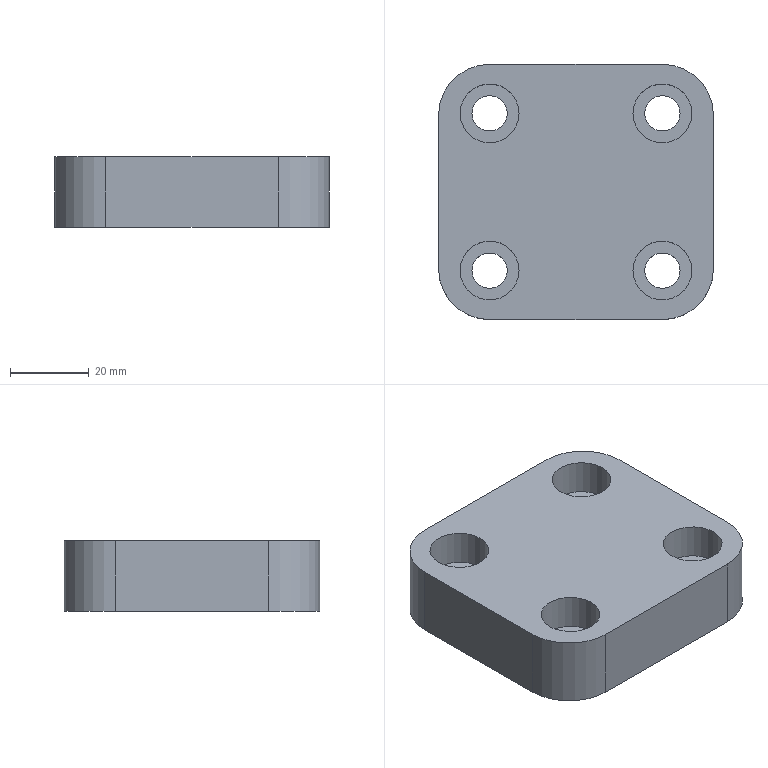Part | STEP file | solid 216 | 1 solid | 22 faces | box 70 x 65 x 18 mm | volume 70637 mm3 | cylinder 12 | plane 10 | commonest cylinder face diameters 9 x4 15 x4 26 x4